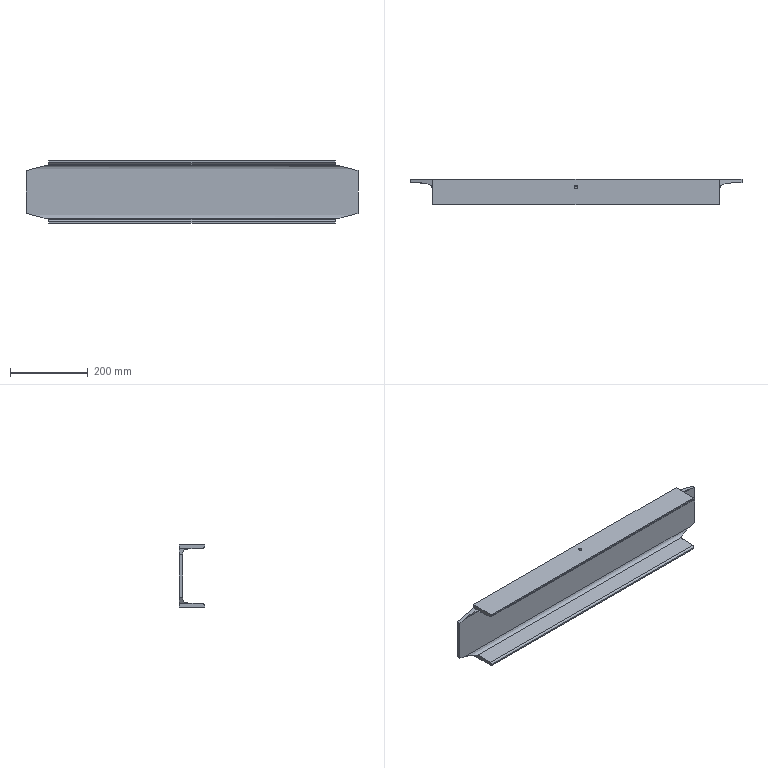Part | STEP file | 05-Channel 160x65_default<machining> | 1 solid | 24 faces | box 853 x 65 x 160 mm | volume 1957806 mm3 | plane 18 | cylinder 6 | commonest cylinder face diameters 8.5 x2 10 x2 20 x2